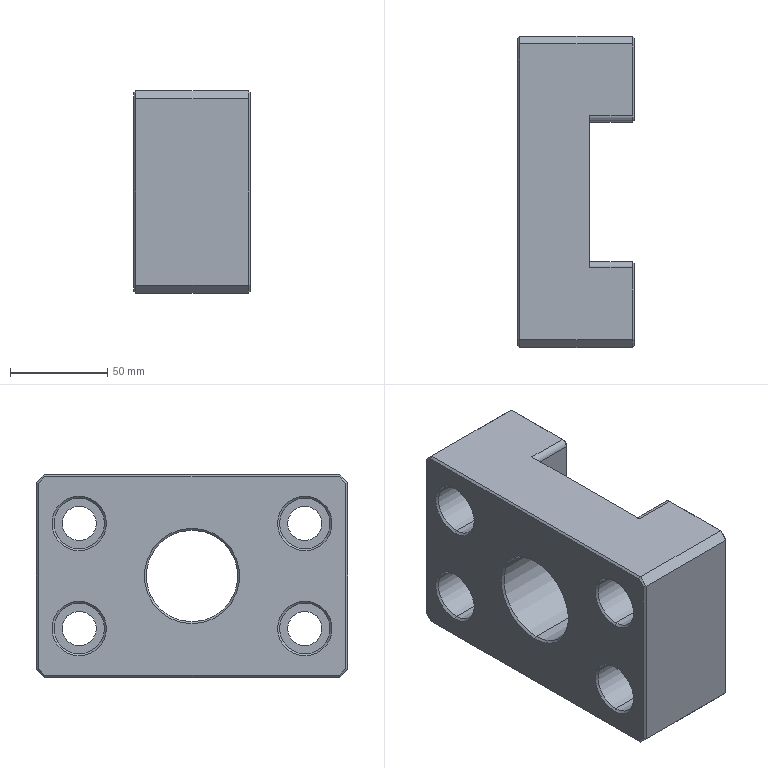Part | STEP file | TJ-DHQM-003-011 | 1 solid | 76 faces | box 60 x 160 x 104 mm | volume 672141 mm3 | plane 38 | cylinder 22 | cone 16 | commonest cylinder face diameters 17.5 x8 26 x8 6 x4 47 x2